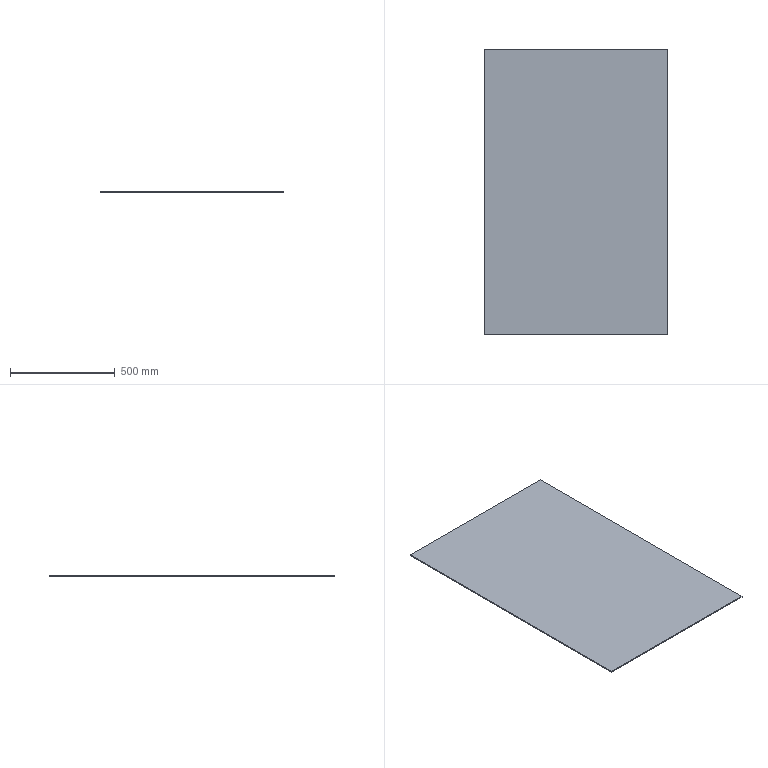Part | SolidWorks | features Extrusion 1, HoleWzd 1 | 1 solid | 6 faces | box 876 x 1360 x 5 mm | volume 5956800 mm3 | plane 6
STEP:
#1=CARTESIAN_POINT('',(438.,-680.,0.));
#2=VERTEX_POINT('',#1);
#3=CARTESIAN_POINT('',(438.,680.,0.));
#4=VERTEX_POINT('',#3);
#5=CARTESIAN_POINT('',(438.,680.,0.));
#6=DIRECTION('',(0.,1.,0.));
#7=VECTOR('',#6,1000.);
#8=LINE('',#5,#7);
#9=EDGE_CURVE('',#2,#4,#8,.T.);
#10=ORIENTED_EDGE('',*,*,#9,.T.);
#11=CARTESIAN_POINT('',(438.,680.,5.));
#12=VERTEX_POINT('',#11);
#13=CARTESIAN_POINT('',(438.,680.,5.));
#14=DIRECTION('',(0.,0.,-1.));
#15=VECTOR('',#14,1000.);
#16=LINE('',#13,#15);
#17=EDGE_CURVE('',#12,#4,#16,.T.);
#18=ORIENTED_EDGE('',*,*,#17,.F.);
#19=CARTESIAN_POINT('',(438.,-680.,5.));
#20=VERTEX_POINT('',#19);
#21=CARTESIAN_POINT('',(438.,680.,5.));
#22=DIRECTION('',(0.,1.,0.));
#23=VECTOR('',#22,1000.);
#24=LINE('',#21,#23);
#25=EDGE_CURVE('',#20,#12,#24,.T.);
#26=ORIENTED_EDGE('',*,*,#25,.F.);
#27=CARTESIAN_POINT('',(438.,-680.,5.));
#28=DIRECTION('',(0.,0.,-1.));
#29=VECTOR('',#28,1000.);
#30=LINE('',#27,#29);
#31=EDGE_CURVE('',#20,#2,#30,.T.);
#32=ORIENTED_EDGE('',*,*,#31,.T.);
#33=EDGE_LOOP('',(#10,#18,#26,#32));
#34=FACE_OUTER_BOUND('',#33,.T.);
#35=CARTESIAN_POINT('',(438.,680.,5.));
#36=DIRECTION('',(-1.,0.,0.));
#37=DIRECTION('',(0.,-1.,0.));
#38=AXIS2_PLACEMENT_3D('',#35,#36,#37);
#39=PLANE('',#38);
#40=ADVANCED_FACE('',(#34),#39,.F.);
#41=CARTESIAN_POINT('',(-438.,680.,0.));
#42=VERTEX_POINT('',#41);
#43=CARTESIAN_POINT('',(-438.,680.,0.));
#44=DIRECTION('',(-1.,0.,0.));
#45=VECTOR('',#44,1000.);
#46=LINE('',#43,#45);
#47=EDGE_CURVE('',#4,#42,#46,.T.);
#48=ORIENTED_EDGE('',*,*,#47,.T.);
#49=CARTESIAN_POINT('',(-438.,680.,5.));
#50=VERTEX_POINT('',#49);
#51=CARTESIAN_POINT('',(-438.,680.,5.));
#52=DIRECTION('',(0.,0.,-1.));
#53=VECTOR('',#52,1000.);
#54=LINE('',#51,#53);
#55=EDGE_CURVE('',#50,#42,#54,.T.);
#56=ORIENTED_EDGE('',*,*,#55,.F.);
#57=CARTESIAN_POINT('',(-438.,680.,5.));
#58=DIRECTION('',(-1.,0.,0.));
#59=VECTOR('',#58,1000.);
#60=LINE('',#57,#59);
#61=EDGE_CURVE('',#12,#50,#60,.T.);
#62=ORIENTED_EDGE('',*,*,#61,.F.);
#63=ORIENTED_EDGE('',*,*,#17,.T.);
#64=EDGE_LOOP('',(#48,#56,#62,#63));
#65=FACE_OUTER_BOUND('',#64,.T.);
#66=CARTESIAN_POINT('',(-438.,680.,5.));
#67=DIRECTION('',(0.,-1.,0.));
#68=DIRECTION('',(0.,0.,-1.));
#69=AXIS2_PLACEMENT_3D('',#66,#67,#68);
#70=PLANE('',#69);
#71=ADVANCED_FACE('',(#65),#70,.F.);
#72=CARTESIAN_POINT('',(-438.,-680.,0.));
#73=VERTEX_POINT('',#72);
#74=CARTESIAN_POINT('',(-438.,680.,0.));
#75=DIRECTION('',(0.,-1.,0.));
#76=VECTOR('',#75,1000.);
#77=LINE('',#74,#76);
#78=EDGE_CURVE('',#42,#73,#77,.T.);
#79=ORIENTED_EDGE('',*,*,#78,.T.);
#80=CARTESIAN_POINT('',(-438.,-680.,5.));
#81=VERTEX_POINT('',#80);
#82=CARTESIAN_POINT('',(-438.,-680.,5.));
#83=DIRECTION('',(0.,0.,-1.));
#84=VECTOR('',#83,1000.);
#85=LINE('',#82,#84);
#86=EDGE_CURVE('',#81,#73,#85,.T.);
#87=ORIENTED_EDGE('',*,*,#86,.F.);
#88=CARTESIAN_POINT('',(-438.,680.,5.));
#89=DIRECTION('',(0.,-1.,0.));
#90=VECTOR('',#89,1000.);
#91=LINE('',#88,#90);
#92=EDGE_CURVE('',#50,#81,#91,.T.);
#93=ORIENTED_EDGE('',*,*,#92,.F.);
#94=ORIENTED_EDGE('',*,*,#55,.T.);
#95=EDGE_LOOP('',(#79,#87,#93,#94));
#96=FACE_OUTER_BOUND('',#95,.T.);
#97=CARTESIAN_POINT('',(-438.,680.,5.));
#98=DIRECTION('',(1.,0.,0.));
#99=DIRECTION('',(0.,1.,0.));
#100=AXIS2_PLACEMENT_3D('',#97,#98,#99);
#101=PLANE('',#100);
#102=ADVANCED_FACE('',(#96),#101,.F.);
#103=CARTESIAN_POINT('',(-438.,-680.,0.));
#104=DIRECTION('',(1.,0.,0.));
#105=VECTOR('',#104,1000.);
#106=LINE('',#103,#105);
#107=EDGE_CURVE('',#73,#2,#106,.T.);
#108=ORIENTED_EDGE('',*,*,#107,.T.);
#109=ORIENTED_EDGE('',*,*,#31,.F.);
#110=CARTESIAN_POINT('',(-438.,-680.,5.));
#111=DIRECTION('',(1.,0.,0.));
#112=VECTOR('',#111,1000.);
#113=LINE('',#110,#112);
#114=EDGE_CURVE('',#81,#20,#113,.T.);
#115=ORIENTED_EDGE('',*,*,#114,.F.);
#116=ORIENTED_EDGE('',*,*,#86,.T.);
#117=EDGE_LOOP('',(#108,#109,#115,#116));
#118=FACE_OUTER_BOUND('',#117,.T.);
#119=CARTESIAN_POINT('',(-438.,-680.,5.));
#120=DIRECTION('',(0.,1.,0.));
#121=DIRECTION('',(0.,0.,1.));
#122=AXIS2_PLACEMENT_3D('',#119,#120,#121);
#123=PLANE('',#122);
#124=ADVANCED_FACE('',(#118),#123,.F.);
#125=ORIENTED_EDGE('',*,*,#25,.T.);
#126=ORIENTED_EDGE('',*,*,#61,.T.);
#127=ORIENTED_EDGE('',*,*,#92,.T.);
#128=ORIENTED_EDGE('',*,*,#114,.T.);
#129=EDGE_LOOP('',(#125,#126,#127,#128));
#130=FACE_OUTER_BOUND('',#129,.T.);
#131=CARTESIAN_POINT('',(0.,0.,5.));
#132=DIRECTION('',(0.,0.,1.));
#133=DIRECTION('',(1.,0.,0.));
#134=AXIS2_PLACEMENT_3D('',#131,#132,#133);
#135=PLANE('',#134);
#136=ADVANCED_FACE('',(#130),#135,.T.);
#137=ORIENTED_EDGE('',*,*,#9,.F.);
#138=ORIENTED_EDGE('',*,*,#107,.F.);
#139=ORIENTED_EDGE('',*,*,#78,.F.);
#140=ORIENTED_EDGE('',*,*,#47,.F.);
#141=EDGE_LOOP('',(#137,#138,#139,#140));
#142=FACE_OUTER_BOUND('',#141,.T.);
#143=CARTESIAN_POINT('',(0.,0.,0.));
#144=DIRECTION('',(0.,0.,1.));
#145=DIRECTION('',(1.,0.,0.));
#146=AXIS2_PLACEMENT_3D('',#143,#144,#145);
#147=PLANE('',#146);
#148=ADVANCED_FACE('',(#142),#147,.F.);
#149=CLOSED_SHELL('',(#40,#71,#102,#124,#136,#148));
#150=MANIFOLD_SOLID_BREP('',#149);
#151=CARTESIAN_POINT('',(0.,0.,0.));
#152=DIRECTION('',(0.,0.,1.));
#153=DIRECTION('',(1.,0.,0.));
#154=AXIS2_PLACEMENT_3D('',#151,#152,#153);
#155=(LENGTH_UNIT()NAMED_UNIT(*)SI_UNIT(.MILLI.,.METRE.));
#156=UNCERTAINTY_MEASURE_WITH_UNIT(LENGTH_MEASURE(0.00001),#155,'','');
#157=(NAMED_UNIT(*)PLANE_ANGLE_UNIT()SI_UNIT($,.RADIAN.));
#158=(NAMED_UNIT(*)SI_UNIT($,.STERADIAN.)SOLID_ANGLE_UNIT());
#159=(GEOMETRIC_REPRESENTATION_CONTEXT(3)GLOBAL_UNCERTAINTY_ASSIGNED_CONTEXT((#156))GLOBAL_UNIT_ASSIGNED_CONTEXT((#155,#157,#158))REPRESENTATION_CONTEXT('',''));
#160=ADVANCED_BREP_SHAPE_REPRESENTATION('',(#150,#154),#159);